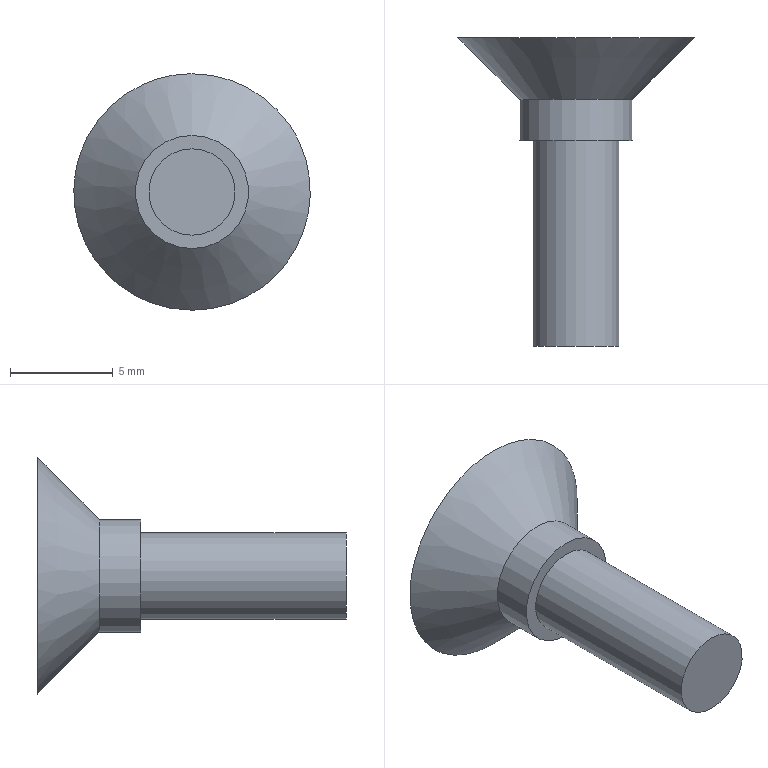Part | STEP file | solid 59 | 1 solid | 6 faces | box 11.5 x 15 x 11.5 mm | volume 365.141 mm3 | plane 2 | cylinder 2 | spline 1 | cone 1 | commonest cylinder face diameters 4.2 x1 5.5 x1